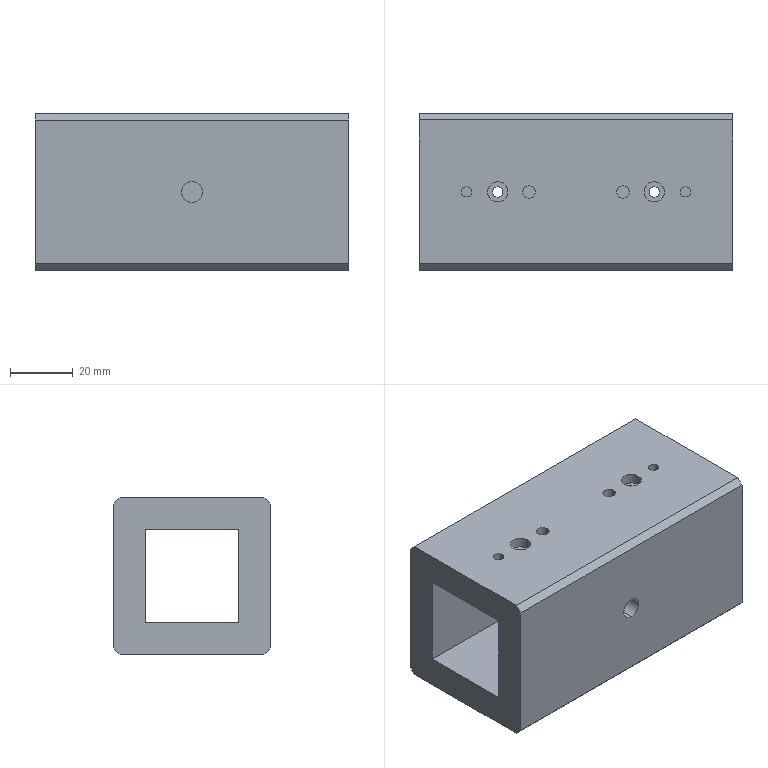Part | SolidWorks | features HoleWzd 7, Chamfer 1, Extrusion 1, ICE 1 | 1 solid | 44 faces | box 100 x 50 x 50 mm | volume 157737 mm3 | cylinder 26 | plane 18 | commonest cylinder face diameters 3.3 x12 6.5 x8 4 x4 6.8 x2
STEP:
#1=CARTESIAN_POINT('',(-26.65,0.,40.));
#2=VERTEX_POINT('',#1);
#3=CARTESIAN_POINT('',(-23.35,0.,40.));
#4=VERTEX_POINT('',#3);
#5=CARTESIAN_POINT('',(-25.,0.,40.));
#6=DIRECTION('',(0.,0.,1.));
#7=DIRECTION('',(0.,-1.,0.));
#8=AXIS2_PLACEMENT_3D('',#5,#6,#7);
#9=CIRCLE('',#8,1.65);
#10=EDGE_CURVE('',#2,#4,#9,.T.);
#11=ORIENTED_EDGE('',*,*,#10,.F.);
#12=CARTESIAN_POINT('',(-26.65,0.,46.6));
#13=VERTEX_POINT('',#12);
#14=CARTESIAN_POINT('',(-26.65,0.,46.6));
#15=DIRECTION('',(0.,0.,1.));
#16=VECTOR('',#15,1000.);
#17=LINE('',#14,#16);
#18=EDGE_CURVE('',#2,#13,#17,.T.);
#19=ORIENTED_EDGE('',*,*,#18,.T.);
#20=CARTESIAN_POINT('',(-23.35,0.,46.6));
#21=VERTEX_POINT('',#20);
#22=CARTESIAN_POINT('',(-25.,0.,46.6));
#23=DIRECTION('',(0.,0.,1.));
#24=DIRECTION('',(1.,0.,0.));
#25=AXIS2_PLACEMENT_3D('',#22,#23,#24);
#26=CIRCLE('',#25,1.65);
#27=EDGE_CURVE('',#13,#21,#26,.T.);
#28=ORIENTED_EDGE('',*,*,#27,.T.);
#29=CARTESIAN_POINT('',(-23.35,0.,46.6));
#30=DIRECTION('',(0.,0.,1.));
#31=VECTOR('',#30,1000.);
#32=LINE('',#29,#31);
#33=EDGE_CURVE('',#4,#21,#32,.T.);
#34=ORIENTED_EDGE('',*,*,#33,.F.);
#35=EDGE_LOOP('',(#11,#19,#28,#34));
#36=FACE_OUTER_BOUND('',#35,.T.);
#37=CARTESIAN_POINT('',(-25.,0.,46.6));
#38=DIRECTION('',(0.,0.,1.));
#39=DIRECTION('',(1.,0.,0.));
#40=AXIS2_PLACEMENT_3D('',#37,#38,#39);
#41=CYLINDRICAL_SURFACE('',#40,1.65);
#42=ADVANCED_FACE('',(#36),#41,.F.);
#43=CARTESIAN_POINT('',(23.35,0.,40.));
#44=VERTEX_POINT('',#43);
#45=CARTESIAN_POINT('',(26.65,0.,40.));
#46=VERTEX_POINT('',#45);
#47=CARTESIAN_POINT('',(25.,0.,40.));
#48=DIRECTION('',(0.,0.,1.));
#49=DIRECTION('',(0.,-1.,0.));
#50=AXIS2_PLACEMENT_3D('',#47,#48,#49);
#51=CIRCLE('',#50,1.65);
#52=EDGE_CURVE('',#44,#46,#51,.T.);
#53=ORIENTED_EDGE('',*,*,#52,.F.);
#54=CARTESIAN_POINT('',(23.35,0.,46.6));
#55=VERTEX_POINT('',#54);
#56=CARTESIAN_POINT('',(23.35,0.,46.6));
#57=DIRECTION('',(0.,0.,1.));
#58=VECTOR('',#57,1000.);
#59=LINE('',#56,#58);
#60=EDGE_CURVE('',#44,#55,#59,.T.);
#61=ORIENTED_EDGE('',*,*,#60,.T.);
#62=CARTESIAN_POINT('',(26.65,0.,46.6));
#63=VERTEX_POINT('',#62);
#64=CARTESIAN_POINT('',(25.,0.,46.6));
#65=DIRECTION('',(0.,0.,1.));
#66=DIRECTION('',(1.,0.,0.));
#67=AXIS2_PLACEMENT_3D('',#64,#65,#66);
#68=CIRCLE('',#67,1.65);
#69=EDGE_CURVE('',#55,#63,#68,.T.);
#70=ORIENTED_EDGE('',*,*,#69,.T.);
#71=CARTESIAN_POINT('',(26.65,0.,46.6));
#72=DIRECTION('',(0.,0.,1.));
#73=VECTOR('',#72,1000.);
#74=LINE('',#71,#73);
#75=EDGE_CURVE('',#46,#63,#74,.T.);
#76=ORIENTED_EDGE('',*,*,#75,.F.);
#77=EDGE_LOOP('',(#53,#61,#70,#76));
#78=FACE_OUTER_BOUND('',#77,.T.);
#79=CARTESIAN_POINT('',(25.,0.,46.6));
#80=DIRECTION('',(0.,0.,1.));
#81=DIRECTION('',(1.,0.,0.));
#82=AXIS2_PLACEMENT_3D('',#79,#80,#81);
#83=CYLINDRICAL_SURFACE('',#82,1.65);
#84=ADVANCED_FACE('',(#78),#83,.F.);
#85=CARTESIAN_POINT('',(26.65,0.,10.));
#86=VERTEX_POINT('',#85);
#87=CARTESIAN_POINT('',(23.35,0.,10.));
#88=VERTEX_POINT('',#87);
#89=CARTESIAN_POINT('',(25.,0.,10.));
#90=DIRECTION('',(0.,0.,-1.));
#91=DIRECTION('',(-1.,0.,0.));
#92=AXIS2_PLACEMENT_3D('',#89,#90,#91);
#93=CIRCLE('',#92,1.65);
#94=EDGE_CURVE('',#86,#88,#93,.T.);
#95=ORIENTED_EDGE('',*,*,#94,.F.);
#96=CARTESIAN_POINT('',(26.65,0.,3.4));
#97=VERTEX_POINT('',#96);
#98=CARTESIAN_POINT('',(26.65,0.,3.4));
#99=DIRECTION('',(0.,0.,-1.));
#100=VECTOR('',#99,1000.);
#101=LINE('',#98,#100);
#102=EDGE_CURVE('',#86,#97,#101,.T.);
#103=ORIENTED_EDGE('',*,*,#102,.T.);
#104=CARTESIAN_POINT('',(23.35,0.,3.4));
#105=VERTEX_POINT('',#104);
#106=CARTESIAN_POINT('',(25.,0.,3.4));
#107=DIRECTION('',(0.,0.,-1.));
#108=DIRECTION('',(-1.,0.,0.));
#109=AXIS2_PLACEMENT_3D('',#106,#107,#108);
#110=CIRCLE('',#109,1.65);
#111=EDGE_CURVE('',#97,#105,#110,.T.);
#112=ORIENTED_EDGE('',*,*,#111,.T.);
#113=CARTESIAN_POINT('',(23.35,0.,3.4));
#114=DIRECTION('',(0.,0.,-1.));
#115=VECTOR('',#114,1000.);
#116=LINE('',#113,#115);
#117=EDGE_CURVE('',#88,#105,#116,.T.);
#118=ORIENTED_EDGE('',*,*,#117,.F.);
#119=EDGE_LOOP('',(#95,#103,#112,#118));
#120=FACE_OUTER_BOUND('',#119,.T.);
#121=CARTESIAN_POINT('',(25.,0.,3.4));
#122=DIRECTION('',(0.,0.,-1.));
#123=DIRECTION('',(-1.,0.,0.));
#124=AXIS2_PLACEMENT_3D('',#121,#122,#123);
#125=CYLINDRICAL_SURFACE('',#124,1.65);
#126=ADVANCED_FACE('',(#120),#125,.F.);
#127=CARTESIAN_POINT('',(-23.35,0.,10.));
#128=VERTEX_POINT('',#127);
#129=CARTESIAN_POINT('',(-26.65,0.,10.));
#130=VERTEX_POINT('',#129);
#131=CARTESIAN_POINT('',(-25.,0.,10.));
#132=DIRECTION('',(0.,0.,-1.));
#133=DIRECTION('',(-1.,0.,0.));
#134=AXIS2_PLACEMENT_3D('',#131,#132,#133);
#135=CIRCLE('',#134,1.65);
#136=EDGE_CURVE('',#128,#130,#135,.T.);
#137=ORIENTED_EDGE('',*,*,#136,.F.);
#138=CARTESIAN_POINT('',(-23.35,0.,3.4));
#139=VERTEX_POINT('',#138);
#140=CARTESIAN_POINT('',(-23.35,0.,3.4));
#141=DIRECTION('',(0.,0.,-1.));
#142=VECTOR('',#141,1000.);
#143=LINE('',#140,#142);
#144=EDGE_CURVE('',#128,#139,#143,.T.);
#145=ORIENTED_EDGE('',*,*,#144,.T.);
#146=CARTESIAN_POINT('',(-26.65,0.,3.4));
#147=VERTEX_POINT('',#146);
#148=CARTESIAN_POINT('',(-25.,0.,3.4));
#149=DIRECTION('',(0.,0.,-1.));
#150=DIRECTION('',(-1.,0.,0.));
#151=AXIS2_PLACEMENT_3D('',#148,#149,#150);
#152=CIRCLE('',#151,1.65);
#153=EDGE_CURVE('',#139,#147,#152,.T.);
#154=ORIENTED_EDGE('',*,*,#153,.T.);
#155=CARTESIAN_POINT('',(-26.65,0.,3.4));
#156=DIRECTION('',(0.,0.,-1.));
#157=VECTOR('',#156,1000.);
#158=LINE('',#155,#157);
#159=EDGE_CURVE('',#130,#147,#158,.T.);
#160=ORIENTED_EDGE('',*,*,#159,.F.);
#161=EDGE_LOOP('',(#137,#145,#154,#160));
#162=FACE_OUTER_BOUND('',#161,.T.);
#163=CARTESIAN_POINT('',(-25.,0.,3.4));
#164=DIRECTION('',(0.,0.,-1.));
#165=DIRECTION('',(-1.,0.,0.));
#166=AXIS2_PLACEMENT_3D('',#163,#164,#165);
#167=CYLINDRICAL_SURFACE('',#166,1.65);
#168=ADVANCED_FACE('',(#162),#167,.F.);
#169=CARTESIAN_POINT('',(0.,-15.,28.4));
#170=VERTEX_POINT('',#169);
#171=CARTESIAN_POINT('',(0.,-15.,21.6));
#172=VERTEX_POINT('',#171);
#173=CARTESIAN_POINT('',(0.,-15.,25.));
#174=DIRECTION('',(0.,-1.,0.));
#175=DIRECTION('',(1.,0.,0.));
#176=AXIS2_PLACEMENT_3D('',#173,#174,#175);
#177=CIRCLE('',#176,3.4);
#178=EDGE_CURVE('',#170,#172,#177,.T.);
#179=ORIENTED_EDGE('',*,*,#178,.F.);
#180=CARTESIAN_POINT('',(0.,-25.,28.4));
#181=VERTEX_POINT('',#180);
#182=CARTESIAN_POINT('',(0.,-25.,28.4));
#183=DIRECTION('',(0.,-1.,0.));
#184=VECTOR('',#183,1000.);
#185=LINE('',#182,#184);
#186=EDGE_CURVE('',#170,#181,#185,.T.);
#187=ORIENTED_EDGE('',*,*,#186,.T.);
#188=CARTESIAN_POINT('',(0.,-25.,21.6));
#189=VERTEX_POINT('',#188);
#190=CARTESIAN_POINT('',(0.,-25.,25.));
#191=DIRECTION('',(0.,-1.,0.));
#192=DIRECTION('',(0.,0.,-1.));
#193=AXIS2_PLACEMENT_3D('',#190,#191,#192);
#194=CIRCLE('',#193,3.4);
#195=EDGE_CURVE('',#181,#189,#194,.T.);
#196=ORIENTED_EDGE('',*,*,#195,.T.);
#197=CARTESIAN_POINT('',(0.,-25.,21.6));
#198=DIRECTION('',(0.,-1.,0.));
#199=VECTOR('',#198,1000.);
#200=LINE('',#197,#199);
#201=EDGE_CURVE('',#172,#189,#200,.T.);
#202=ORIENTED_EDGE('',*,*,#201,.F.);
#203=EDGE_LOOP('',(#179,#187,#196,#202));
#204=FACE_OUTER_BOUND('',#203,.T.);
#205=CARTESIAN_POINT('',(0.,-25.,25.));
#206=DIRECTION('',(0.,-1.,0.));
#207=DIRECTION('',(0.,0.,-1.));
#208=AXIS2_PLACEMENT_3D('',#205,#206,#207);
#209=CYLINDRICAL_SURFACE('',#208,3.4);
#210=ADVANCED_FACE('',(#204),#209,.F.);
#211=CARTESIAN_POINT('',(13.,0.,40.));
#212=VERTEX_POINT('',#211);
#213=CARTESIAN_POINT('',(17.,0.,40.));
#214=VERTEX_POINT('',#213);
#215=CARTESIAN_POINT('',(15.,0.,40.));
#216=DIRECTION('',(0.,0.,1.));
#217=DIRECTION('',(0.,-1.,0.));
#218=AXIS2_PLACEMENT_3D('',#215,#216,#217);
#219=CIRCLE('',#218,2.);
#220=EDGE_CURVE('',#212,#214,#219,.T.);
#221=ORIENTED_EDGE('',*,*,#220,.F.);
#222=CARTESIAN_POINT('',(13.,0.,50.));
#223=VERTEX_POINT('',#222);
#224=CARTESIAN_POINT('',(13.,0.,50.));
#225=DIRECTION('',(0.,0.,1.));
#226=VECTOR('',#225,1000.);
#227=LINE('',#224,#226);
#228=EDGE_CURVE('',#212,#223,#227,.T.);
#229=ORIENTED_EDGE('',*,*,#228,.T.);
#230=CARTESIAN_POINT('',(17.,0.,50.));
#231=VERTEX_POINT('',#230);
#232=CARTESIAN_POINT('',(15.,0.,50.));
#233=DIRECTION('',(0.,0.,1.));
#234=DIRECTION('',(1.,0.,0.));
#235=AXIS2_PLACEMENT_3D('',#232,#233,#234);
#236=CIRCLE('',#235,2.);
#237=EDGE_CURVE('',#223,#231,#236,.T.);
#238=ORIENTED_EDGE('',*,*,#237,.T.);
#239=CARTESIAN_POINT('',(17.,0.,50.));
#240=DIRECTION('',(0.,0.,1.));
#241=VECTOR('',#240,1000.);
#242=LINE('',#239,#241);
#243=EDGE_CURVE('',#214,#231,#242,.T.);
#244=ORIENTED_EDGE('',*,*,#243,.F.);
#245=EDGE_LOOP('',(#221,#229,#238,#244));
#246=FACE_OUTER_BOUND('',#245,.T.);
#247=CARTESIAN_POINT('',(15.,0.,50.));
#248=DIRECTION('',(0.,0.,1.));
#249=DIRECTION('',(1.,0.,0.));
#250=AXIS2_PLACEMENT_3D('',#247,#248,#249);
#251=CYLINDRICAL_SURFACE('',#250,2.);
#252=ADVANCED_FACE('',(#246),#251,.F.);
#253=CARTESIAN_POINT('',(-17.,0.,40.));
#254=VERTEX_POINT('',#253);
#255=CARTESIAN_POINT('',(-13.,0.,40.));
#256=VERTEX_POINT('',#255);
#257=CARTESIAN_POINT('',(-15.,0.,40.));
#258=DIRECTION('',(0.,0.,1.));
#259=DIRECTION('',(0.,-1.,0.));
#260=AXIS2_PLACEMENT_3D('',#257,#258,#259);
#261=CIRCLE('',#260,2.);
#262=EDGE_CURVE('',#254,#256,#261,.T.);
#263=ORIENTED_EDGE('',*,*,#262,.F.);
#264=CARTESIAN_POINT('',(-17.,0.,50.));
#265=VERTEX_POINT('',#264);
#266=CARTESIAN_POINT('',(-17.,0.,50.));
#267=DIRECTION('',(0.,0.,1.));
#268=VECTOR('',#267,1000.);
#269=LINE('',#266,#268);
#270=EDGE_CURVE('',#254,#265,#269,.T.);
#271=ORIENTED_EDGE('',*,*,#270,.T.);
#272=CARTESIAN_POINT('',(-13.,0.,50.));
#273=VERTEX_POINT('',#272);
#274=CARTESIAN_POINT('',(-15.,0.,50.));
#275=DIRECTION('',(0.,0.,1.));
#276=DIRECTION('',(1.,0.,0.));
#277=AXIS2_PLACEMENT_3D('',#274,#275,#276);
#278=CIRCLE('',#277,2.);
#279=EDGE_CURVE('',#265,#273,#278,.T.);
#280=ORIENTED_EDGE('',*,*,#279,.T.);
#281=CARTESIAN_POINT('',(-13.,0.,50.));
#282=DIRECTION('',(0.,0.,1.));
#283=VECTOR('',#282,1000.);
#284=LINE('',#281,#283);
#285=EDGE_CURVE('',#256,#273,#284,.T.);
#286=ORIENTED_EDGE('',*,*,#285,.F.);
#287=EDGE_LOOP('',(#263,#271,#280,#286));
#288=FACE_OUTER_BOUND('',#287,.T.);
#289=CARTESIAN_POINT('',(-15.,0.,50.));
#290=DIRECTION('',(0.,0.,1.));
#291=DIRECTION('',(1.,0.,0.));
#292=AXIS2_PLACEMENT_3D('',#289,#290,#291);
#293=CYLINDRICAL_SURFACE('',#292,2.);
#294=ADVANCED_FACE('',(#288),#293,.F.);
#295=CARTESIAN_POINT('',(-36.65,0.,40.));
#296=VERTEX_POINT('',#295);
#297=CARTESIAN_POINT('',(-33.35,0.,40.));
#298=VERTEX_POINT('',#297);
#299=CARTESIAN_POINT('',(-35.,0.,40.));
#300=DIRECTION('',(0.,0.,1.));
#301=DIRECTION('',(0.,-1.,0.));
#302=AXIS2_PLACEMENT_3D('',#299,#300,#301);
#303=CIRCLE('',#302,1.65);
#304=EDGE_CURVE('',#296,#298,#303,.T.);
#305=ORIENTED_EDGE('',*,*,#304,.F.);
#306=CARTESIAN_POINT('',(-36.65,0.,50.));
#307=VERTEX_POINT('',#306);
#308=CARTESIAN_POINT('',(-36.65,0.,50.));
#309=DIRECTION('',(0.,0.,1.));
#310=VECTOR('',#309,1000.);
#311=LINE('',#308,#310);
#312=EDGE_CURVE('',#296,#307,#311,.T.);
#313=ORIENTED_EDGE('',*,*,#312,.T.);
#314=CARTESIAN_POINT('',(-33.35,0.,50.));
#315=VERTEX_POINT('',#314);
#316=CARTESIAN_POINT('',(-35.,0.,50.));
#317=DIRECTION('',(0.,0.,1.));
#318=DIRECTION('',(1.,0.,0.));
#319=AXIS2_PLACEMENT_3D('',#316,#317,#318);
#320=CIRCLE('',#319,1.65);
#321=EDGE_CURVE('',#307,#315,#320,.T.);
#322=ORIENTED_EDGE('',*,*,#321,.T.);
#323=CARTESIAN_POINT('',(-33.35,0.,50.));
#324=DIRECTION('',(0.,0.,1.));
#325=VECTOR('',#324,1000.);
#326=LINE('',#323,#325);
#327=EDGE_CURVE('',#298,#315,#326,.T.);
#328=ORIENTED_EDGE('',*,*,#327,.F.);
#329=EDGE_LOOP('',(#305,#313,#322,#328));
#330=FACE_OUTER_BOUND('',#329,.T.);
#331=CARTESIAN_POINT('',(-35.,0.,50.));
#332=DIRECTION('',(0.,0.,1.));
#333=DIRECTION('',(1.,0.,0.));
#334=AXIS2_PLACEMENT_3D('',#331,#332,#333);
#335=CYLINDRICAL_SURFACE('',#334,1.65);
#336=ADVANCED_FACE('',(#330),#335,.F.);
#337=CARTESIAN_POINT('',(33.35,0.,40.));
#338=VERTEX_POINT('',#337);
#339=CARTESIAN_POINT('',(36.65,0.,40.));
#340=VERTEX_POINT('',#339);
#341=CARTESIAN_POINT('',(35.,0.,40.));
#342=DIRECTION('',(0.,0.,1.));
#343=DIRECTION('',(0.,-1.,0.));
#344=AXIS2_PLACEMENT_3D('',#341,#342,#343);
#345=CIRCLE('',#344,1.65);
#346=EDGE_CURVE('',#338,#340,#345,.T.);
#347=ORIENTED_EDGE('',*,*,#346,.F.);
#348=CARTESIAN_POINT('',(33.35,0.,50.));
#349=VERTEX_POINT('',#348);
#350=CARTESIAN_POINT('',(33.35,0.,50.));
#351=DIRECTION('',(0.,0.,1.));
#352=VECTOR('',#351,1000.);
#353=LINE('',#350,#352);
#354=EDGE_CURVE('',#338,#349,#353,.T.);
#355=ORIENTED_EDGE('',*,*,#354,.T.);
#356=CARTESIAN_POINT('',(36.65,0.,50.));
#357=VERTEX_POINT('',#356);
#358=CARTESIAN_POINT('',(35.,0.,50.));
#359=DIRECTION('',(0.,0.,1.));
#360=DIRECTION('',(1.,0.,0.));
#361=AXIS2_PLACEMENT_3D('',#358,#359,#360);
#362=CIRCLE('',#361,1.65);
#363=EDGE_CURVE('',#349,#357,#362,.T.);
#364=ORIENTED_EDGE('',*,*,#363,.T.);
#365=CARTESIAN_POINT('',(36.65,0.,50.));
#366=DIRECTION('',(0.,0.,1.));
#367=VECTOR('',#366,1000.);
#368=LINE('',#365,#367);
#369=EDGE_CURVE('',#340,#357,#368,.T.);
#370=ORIENTED_EDGE('',*,*,#369,.F.);
#371=EDGE_LOOP('',(#347,#355,#364,#370));
#372=FACE_OUTER_BOUND('',#371,.T.);
#373=CARTESIAN_POINT('',(35.,0.,50.));
#374=DIRECTION('',(0.,0.,1.));
#375=DIRECTION('',(1.,0.,0.));
#376=AXIS2_PLACEMENT_3D('',#373,#374,#375);
#377=CYLINDRICAL_SURFACE('',#376,1.65);
#378=ADVANCED_FACE('',(#372),#377,.F.);
#379=CARTESIAN_POINT('',(-28.25,0.,46.6));
#380=VERTEX_POINT('',#379);
#381=CARTESIAN_POINT('',(-21.75,0.,46.6));
#382=VERTEX_POINT('',#381);
#383=CARTESIAN_POINT('',(-25.,0.,46.6));
#384=DIRECTION('',(0.,0.,1.));
#385=DIRECTION('',(1.,0.,0.));
#386=AXIS2_PLACEMENT_3D('',#383,#384,#385);
#387=CIRCLE('',#386,3.25);
#388=EDGE_CURVE('',#380,#382,#387,.T.);
#389=ORIENTED_EDGE('',*,*,#388,.F.);
#390=CARTESIAN_POINT('',(-28.25,0.,50.));
#391=VERTEX_POINT('',#390);
#392=CARTESIAN_POINT('',(-28.25,0.,50.));
#393=DIRECTION('',(0.,0.,1.));
#394=VECTOR('',#393,1000.);
#395=LINE('',#392,#394);
#396=EDGE_CURVE('',#380,#391,#395,.T.);
#397=ORIENTED_EDGE('',*,*,#396,.T.);
#398=CARTESIAN_POINT('',(-21.75,0.,50.));
#399=VERTEX_POINT('',#398);
#400=CARTESIAN_POINT('',(-25.,0.,50.));
#401=DIRECTION('',(0.,0.,1.));
#402=DIRECTION('',(1.,0.,0.));
#403=AXIS2_PLACEMENT_3D('',#400,#401,#402);
#404=CIRCLE('',#403,3.25);
#405=EDGE_CURVE('',#391,#399,#404,.T.);
#406=ORIENTED_EDGE('',*,*,#405,.T.);
#407=CARTESIAN_POINT('',(-21.75,0.,50.));
#408=DIRECTION('',(0.,0.,1.));
#409=VECTOR('',#408,1000.);
#410=LINE('',#407,#409);
#411=EDGE_CURVE('',#382,#399,#410,.T.);
#412=ORIENTED_EDGE('',*,*,#411,.F.);
#413=EDGE_LOOP('',(#389,#397,#406,#412));
#414=FACE_OUTER_BOUND('',#413,.T.);
#415=CARTESIAN_POINT('',(-25.,0.,50.));
#416=DIRECTION('',(0.,0.,1.));
#417=DIRECTION('',(1.,0.,0.));
#418=AXIS2_PLACEMENT_3D('',#415,#416,#417);
#419=CYLINDRICAL_SURFACE('',#418,3.25);
#420=ADVANCED_FACE('',(#414),#419,.F.);
#421=CARTESIAN_POINT('',(21.75,0.,46.6));
#422=VERTEX_POINT('',#421);
#423=CARTESIAN_POINT('',(28.25,0.,46.6));
#424=VERTEX_POINT('',#423);
#425=CARTESIAN_POINT('',(25.,0.,46.6));
#426=DIRECTION('',(0.,0.,1.));
#427=DIRECTION('',(1.,0.,0.));
#428=AXIS2_PLACEMENT_3D('',#425,#426,#427);
#429=CIRCLE('',#428,3.25);
#430=EDGE_CURVE('',#422,#424,#429,.T.);
#431=ORIENTED_EDGE('',*,*,#430,.F.);
#432=CARTESIAN_POINT('',(21.75,0.,50.));
#433=VERTEX_POINT('',#432);
#434=CARTESIAN_POINT('',(21.75,0.,50.));
#435=DIRECTION('',(0.,0.,1.));
#436=VECTOR('',#435,1000.);
#437=LINE('',#434,#436);
#438=EDGE_CURVE('',#422,#433,#437,.T.);
#439=ORIENTED_EDGE('',*,*,#438,.T.);
#440=CARTESIAN_POINT('',(28.25,0.,50.));
#441=VERTEX_POINT('',#440);
#442=CARTESIAN_POINT('',(25.,0.,50.));
#443=DIRECTION('',(0.,0.,1.));
#444=DIRECTION('',(1.,0.,0.));
#445=AXIS2_PLACEMENT_3D('',#442,#443,#444);
#446=CIRCLE('',#445,3.25);
#447=EDGE_CURVE('',#433,#441,#446,.T.);
#448=ORIENTED_EDGE('',*,*,#447,.T.);
#449=CARTESIAN_POINT('',(28.25,0.,50.));
#450=DIRECTION('',(0.,0.,1.));
#451=VECTOR('',#450,1000.);
#452=LINE('',#449,#451);
#453=EDGE_CURVE('',#424,#441,#452,.T.);
#454=ORIENTED_EDGE('',*,*,#453,.F.);
#455=EDGE_LOOP('',(#431,#439,#448,#454));
#456=FACE_OUTER_BOUND('',#455,.T.);
#457=CARTESIAN_POINT('',(25.,0.,50.));
#458=DIRECTION('',(0.,0.,1.));
#459=DIRECTION('',(1.,0.,0.));
#460=AXIS2_PLACEMENT_3D('',#457,#458,#459);
#461=CYLINDRICAL_SURFACE('',#460,3.25);
#462=ADVANCED_FACE('',(#456),#461,.F.);
#463=CARTESIAN_POINT('',(28.25,0.,3.4));
#464=VERTEX_POINT('',#463);
#465=CARTESIAN_POINT('',(21.75,0.,3.4));
#466=VERTEX_POINT('',#465);
#467=CARTESIAN_POINT('',(25.,0.,3.4));
#468=DIRECTION('',(0.,0.,-1.));
#469=DIRECTION('',(-1.,0.,0.));
#470=AXIS2_PLACEMENT_3D('',#467,#468,#469);
#471=CIRCLE('',#470,3.25);
#472=EDGE_CURVE('',#464,#466,#471,.T.);
#473=ORIENTED_EDGE('',*,*,#472,.F.);
#474=CARTESIAN_POINT('',(28.25,0.,0.));
#475=VERTEX_POINT('',#474);
#476=CARTESIAN_POINT('',(28.25,0.,0.));
#477=DIRECTION('',(0.,0.,-1.));
#478=VECTOR('',#477,1000.);
#479=LINE('',#476,#478);
#480=EDGE_CURVE('',#464,#475,#479,.T.);
#481=ORIENTED_EDGE('',*,*,#480,.T.);
#482=CARTESIAN_POINT('',(21.75,0.,0.));
#483=VERTEX_POINT('',#482);
#484=CARTESIAN_POINT('',(25.,0.,0.));
#485=DIRECTION('',(0.,0.,-1.));
#486=DIRECTION('',(-1.,0.,0.));
#487=AXIS2_PLACEMENT_3D('',#484,#485,#486);
#488=CIRCLE('',#487,3.25);
#489=EDGE_CURVE('',#475,#483,#488,.T.);
#490=ORIENTED_EDGE('',*,*,#489,.T.);
#491=CARTESIAN_POINT('',(21.75,0.,0.));
#492=DIRECTION('',(0.,0.,-1.));
#493=VECTOR('',#492,1000.);
#494=LINE('',#491,#493);
#495=EDGE_CURVE('',#466,#483,#494,.T.);
#496=ORIENTED_EDGE('',*,*,#495,.F.);
#497=EDGE_LOOP('',(#473,#481,#490,#496));
#498=FACE_OUTER_BOUND('',#497,.T.);
#499=CARTESIAN_POINT('',(25.,0.,0.));
#500=DIRECTION('',(0.,0.,-1.));
#501=DIRECTION('',(-1.,0.,0.));
#502=AXIS2_PLACEMENT_3D('',#499,#500,#501);
#503=CYLINDRICAL_SURFACE('',#502,3.25);
#504=ADVANCED_FACE('',(#498),#503,.F.);
#505=CARTESIAN_POINT('',(-21.75,0.,3.4));
#506=VERTEX_POINT('',#505);
#507=CARTESIAN_POINT('',(-28.25,0.,3.4));
#508=VERTEX_POINT('',#507);
#509=CARTESIAN_POINT('',(-25.,0.,3.4));
#510=DIRECTION('',(0.,0.,-1.));
#511=DIRECTION('',(-1.,0.,0.));
#512=AXIS2_PLACEMENT_3D('',#509,#510,#511);
#513=CIRCLE('',#512,3.25);
#514=EDGE_CURVE('',#506,#508,#513,.T.);
#515=ORIENTED_EDGE('',*,*,#514,.F.);
#516=CARTESIAN_POINT('',(-21.75,0.,0.));
#517=VERTEX_POINT('',#516);
#518=CARTESIAN_POINT('',(-21.75,0.,0.));
#519=DIRECTION('',(0.,0.,-1.));
#520=VECTOR('',#519,1000.);
#521=LINE('',#518,#520);
#522=EDGE_CURVE('',#506,#517,#521,.T.);
#523=ORIENTED_EDGE('',*,*,#522,.T.);
#524=CARTESIAN_POINT('',(-28.25,0.,0.));
#525=VERTEX_POINT('',#524);
#526=CARTESIAN_POINT('',(-25.,0.,0.));
#527=DIRECTION('',(0.,0.,-1.));
#528=DIRECTION('',(-1.,0.,0.));
#529=AXIS2_PLACEMENT_3D('',#526,#527,#528);
#530=CIRCLE('',#529,3.25);
#531=EDGE_CURVE('',#517,#525,#530,.T.);
#532=ORIENTED_EDGE('',*,*,#531,.T.);
#533=CARTESIAN_POINT('',(-28.25,0.,0.));
#534=DIRECTION('',(0.,0.,-1.));
#535=VECTOR('',#534,1000.);
#536=LINE('',#533,#535);
#537=EDGE_CURVE('',#508,#525,#536,.T.);
#538=ORIENTED_EDGE('',*,*,#537,.F.);
#539=EDGE_LOOP('',(#515,#523,#532,#538));
#540=FACE_OUTER_BOUND('',#539,.T.);
#541=CARTESIAN_POINT('',(-25.,0.,0.));
#542=DIRECTION('',(0.,0.,-1.));
#543=DIRECTION('',(-1.,0.,0.));
#544=AXIS2_PLACEMENT_3D('',#541,#542,#543);
#545=CYLINDRICAL_SURFACE('',#544,3.25);
#546=ADVANCED_FACE('',(#540),#545,.F.);
#547=CARTESIAN_POINT('',(50.,-15.,40.));
#548=VERTEX_POINT('',#547);
#549=CARTESIAN_POINT('',(50.,-15.,10.));
#550=VERTEX_POINT('',#549);
#551=CARTESIAN_POINT('',(50.,-15.,40.));
#552=DIRECTION('',(0.,0.,-1.));
#553=VECTOR('',#552,1000.);
#554=LINE('',#551,#553);
#555=EDGE_CURVE('',#548,#550,#554,.T.);
#556=ORIENTED_EDGE('',*,*,#555,.F.);
#557=CARTESIAN_POINT('',(50.,15.,40.));
#558=VERTEX_POINT('',#557);
#559=CARTESIAN_POINT('',(50.,15.,40.));
#560=DIRECTION('',(0.,-1.,0.));
#561=VECTOR('',#560,1000.);
#562=LINE('',#559,#561);
#563=EDGE_CURVE('',#558,#548,#562,.T.);
#564=ORIENTED_EDGE('',*,*,#563,.F.);
#565=CARTESIAN_POINT('',(50.,15.,10.));
#566=VERTEX_POINT('',#565);
#567=CARTESIAN_POINT('',(50.,15.,40.));
#568=DIRECTION('',(0.,0.,1.));
#569=VECTOR('',#568,1000.);
#570=LINE('',#567,#569);
#571=EDGE_CURVE('',#566,#558,#570,.T.);
#572=ORIENTED_EDGE('',*,*,#571,.F.);
#573=CARTESIAN_POINT('',(50.,15.,10.));
#574=DIRECTION('',(0.,1.,0.));
#575=VECTOR('',#574,1000.);
#576=LINE('',#573,#575);
#577=EDGE_CURVE('',#550,#566,#576,.T.);
#578=ORIENTED_EDGE('',*,*,#577,.F.);
#579=EDGE_LOOP('',(#556,#564,#572,#578));
#580=FACE_BOUND('',#579,.T.);
#581=CARTESIAN_POINT('',(50.,-23.,50.));
#582=VERTEX_POINT('',#581);
#583=CARTESIAN_POINT('',(50.,23.,50.));
#584=VERTEX_POINT('',#583);
#585=CARTESIAN_POINT('',(50.,25.,50.));
#586=DIRECTION('',(0.,1.,0.));
#587=VECTOR('',#586,1000.);
#588=LINE('',#585,#587);
#589=EDGE_CURVE('',#582,#584,#588,.T.);
#590=ORIENTED_EDGE('',*,*,#589,.F.);
#591=CARTESIAN_POINT('',(50.,-25.,48.));
#592=VERTEX_POINT('',#591);
#593=CARTESIAN_POINT('',(50.,-23.,50.));
#594=DIRECTION('',(0.,-0.7071,-0.7071));
#595=VECTOR('',#594,1000.);
#596=LINE('',#593,#595);
#597=EDGE_CURVE('',#582,#592,#596,.T.);
#598=ORIENTED_EDGE('',*,*,#597,.T.);
#599=CARTESIAN_POINT('',(50.,-25.,2.));
#600=VERTEX_POINT('',#599);
#601=CARTESIAN_POINT('',(50.,-25.,50.));
#602=DIRECTION('',(0.,0.,-1.));
#603=VECTOR('',#602,1000.);
#604=LINE('',#601,#603);
#605=EDGE_CURVE('',#592,#600,#604,.T.);
#606=ORIENTED_EDGE('',*,*,#605,.T.);
#607=CARTESIAN_POINT('',(50.,-23.,0.));
#608=VERTEX_POINT('',#607);
#609=CARTESIAN_POINT('',(50.,-25.,2.));
#610=DIRECTION('',(0.,0.7071,-0.7071));
#611=VECTOR('',#610,1000.);
#612=LINE('',#609,#611);
#613=EDGE_CURVE('',#600,#608,#612,.T.);
#614=ORIENTED_EDGE('',*,*,#613,.T.);
#615=CARTESIAN_POINT('',(50.,23.,0.));
#616=VERTEX_POINT('',#615);
#617=CARTESIAN_POINT('',(50.,25.,0.));
#618=DIRECTION('',(0.,1.,0.));
#619=VECTOR('',#618,1000.);
#620=LINE('',#617,#619);
#621=EDGE_CURVE('',#608,#616,#620,.T.);
#622=ORIENTED_EDGE('',*,*,#621,.T.);
#623=CARTESIAN_POINT('',(50.,25.,2.));
#624=VERTEX_POINT('',#623);
#625=CARTESIAN_POINT('',(50.,25.,2.));
#626=DIRECTION('',(0.,0.7071,0.7071));
#627=VECTOR('',#626,1000.);
#628=LINE('',#625,#627);
#629=EDGE_CURVE('',#616,#624,#628,.T.);
#630=ORIENTED_EDGE('',*,*,#629,.T.);
#631=CARTESIAN_POINT('',(50.,25.,48.));
#632=VERTEX_POINT('',#631);
#633=CARTESIAN_POINT('',(50.,25.,50.));
#634=DIRECTION('',(0.,0.,-1.));
#635=VECTOR('',#634,1000.);
#636=LINE('',#633,#635);
#637=EDGE_CURVE('',#632,#624,#636,.T.);
#638=ORIENTED_EDGE('',*,*,#637,.F.);
#639=CARTESIAN_POINT('',(50.,23.,50.));
#640=DIRECTION('',(0.,-0.7071,0.7071));
#641=VECTOR('',#640,1000.);
#642=LINE('',#639,#641);
#643=EDGE_CURVE('',#632,#584,#642,.T.);
#644=ORIENTED_EDGE('',*,*,#643,.T.);
#645=EDGE_LOOP('',(#590,#598,#606,#614,#622,#630,#638,#644));
#646=FACE_OUTER_BOUND('',#645,.T.);
#647=CARTESIAN_POINT('',(50.,25.,50.));
#648=DIRECTION('',(-1.,0.,0.));
#649=DIRECTION('',(0.,0.,1.));
#650=AXIS2_PLACEMENT_3D('',#647,#648,#649);
#651=PLANE('',#650);
#652=ADVANCED_FACE('',(#580,#646),#651,.F.);
#653=CARTESIAN_POINT('',(-50.,25.,48.));
#654=VERTEX_POINT('',#653);
#655=CARTESIAN_POINT('',(-50.,25.,2.));
#656=VERTEX_POINT('',#655);
#657=CARTESIAN_POINT('',(-50.,25.,50.));
#658=DIRECTION('',(0.,0.,-1.));
#659=VECTOR('',#658,1000.);
#660=LINE('',#657,#659);
#661=EDGE_CURVE('',#654,#656,#660,.T.);
#662=ORIENTED_EDGE('',*,*,#661,.F.);
#663=CARTESIAN_POINT('',(50.,25.,48.));
#664=DIRECTION('',(1.,0.,0.));
#665=VECTOR('',#664,1000.);
#666=LINE('',#663,#665);
#667=EDGE_CURVE('',#654,#632,#666,.T.);
#668=ORIENTED_EDGE('',*,*,#667,.T.);
#669=ORIENTED_EDGE('',*,*,#637,.T.);
#670=CARTESIAN_POINT('',(-50.,25.,2.));
#671=DIRECTION('',(-1.,0.,0.));
#672=VECTOR('',#671,1000.);
#673=LINE('',#670,#672);
#674=EDGE_CURVE('',#624,#656,#673,.T.);
#675=ORIENTED_EDGE('',*,*,#674,.T.);
#676=EDGE_LOOP('',(#662,#668,#669,#675));
#677=FACE_OUTER_BOUND('',#676,.T.);
#678=CARTESIAN_POINT('',(-50.,25.,50.));
#679=DIRECTION('',(0.,-1.,0.));
#680=DIRECTION('',(0.,0.,-1.));
#681=AXIS2_PLACEMENT_3D('',#678,#679,#680);
#682=PLANE('',#681);
#683=ADVANCED_FACE('',(#677),#682,.F.);
#684=CARTESIAN_POINT('',(-50.,15.,10.));
#685=VERTEX_POINT('',#684);
#686=CARTESIAN_POINT('',(-50.,15.,40.));
#687=VERTEX_POINT('',#686);
#688=CARTESIAN_POINT('',(-50.,15.,40.));
#689=DIRECTION('',(0.,0.,1.));
#690=VECTOR('',#689,1000.);
#691=LINE('',#688,#690);
#692=EDGE_CURVE('',#685,#687,#691,.T.);
#693=ORIENTED_EDGE('',*,*,#692,.T.);
#694=CARTESIAN_POINT('',(-50.,-15.,40.));
#695=VERTEX_POINT('',#694);
#696=CARTESIAN_POINT('',(-50.,15.,40.));
#697=DIRECTION('',(0.,-1.,0.));
#698=VECTOR('',#697,1000.);
#699=LINE('',#696,#698);
#700=EDGE_CURVE('',#687,#695,#699,.T.);
#701=ORIENTED_EDGE('',*,*,#700,.T.);
#702=CARTESIAN_POINT('',(-50.,-15.,10.));
#703=VERTEX_POINT('',#702);
#704=CARTESIAN_POINT('',(-50.,-15.,40.));
#705=DIRECTION('',(0.,0.,-1.));
#706=VECTOR('',#705,1000.);
#707=LINE('',#704,#706);
#708=EDGE_CURVE('',#695,#703,#707,.T.);
#709=ORIENTED_EDGE('',*,*,#708,.T.);
#710=CARTESIAN_POINT('',(-50.,15.,10.));
#711=DIRECTION('',(0.,1.,0.));
#712=VECTOR('',#711,1000.);
#713=LINE('',#710,#712);
#714=EDGE_CURVE('',#703,#685,#713,.T.);
#715=ORIENTED_EDGE('',*,*,#714,.T.);
#716=EDGE_LOOP('',(#693,#701,#709,#715));
#717=FACE_BOUND('',#716,.T.);
#718=CARTESIAN_POINT('',(-50.,-25.,48.));
#719=VERTEX_POINT('',#718);
#720=CARTESIAN_POINT('',(-50.,-25.,2.));
#721=VERTEX_POINT('',#720);
#722=CARTESIAN_POINT('',(-50.,-25.,50.));
#723=DIRECTION('',(0.,0.,-1.));
#724=VECTOR('',#723,1000.);
#725=LINE('',#722,#724);
#726=EDGE_CURVE('',#719,#721,#725,.T.);
#727=ORIENTED_EDGE('',*,*,#726,.F.);
#728=CARTESIAN_POINT('',(-50.,-23.,50.));
#729=VERTEX_POINT('',#728);
#730=CARTESIAN_POINT('',(-50.,-23.,50.));
#731=DIRECTION('',(0.,0.7071,0.7071));
#732=VECTOR('',#731,1000.);
#733=LINE('',#730,#732);
#734=EDGE_CURVE('',#719,#729,#733,.T.);
#735=ORIENTED_EDGE('',*,*,#734,.T.);
#736=CARTESIAN_POINT('',(-50.,23.,50.));
#737=VERTEX_POINT('',#736);
#738=CARTESIAN_POINT('',(-50.,25.,50.));
#739=DIRECTION('',(0.,-1.,0.));
#740=VECTOR('',#739,1000.);
#741=LINE('',#738,#740);
#742=EDGE_CURVE('',#737,#729,#741,.T.);
#743=ORIENTED_EDGE('',*,*,#742,.F.);
#744=CARTESIAN_POINT('',(-50.,23.,50.));
#745=DIRECTION('',(0.,0.7071,-0.7071));
#746=VECTOR('',#745,1000.);
#747=LINE('',#744,#746);
#748=EDGE_CURVE('',#737,#654,#747,.T.);
#749=ORIENTED_EDGE('',*,*,#748,.T.);
#750=ORIENTED_EDGE('',*,*,#661,.T.);
#751=CARTESIAN_POINT('',(-50.,23.,0.));
#752=VERTEX_POINT('',#751);
#753=CARTESIAN_POINT('',(-50.,25.,2.));
#754=DIRECTION('',(0.,-0.7071,-0.7071));
#755=VECTOR('',#754,1000.);
#756=LINE('',#753,#755);
#757=EDGE_CURVE('',#656,#752,#756,.T.);
#758=ORIENTED_EDGE('',*,*,#757,.T.);
#759=CARTESIAN_POINT('',(-50.,-23.,0.));
#760=VERTEX_POINT('',#759);
#761=CARTESIAN_POINT('',(-50.,25.,0.));
#762=DIRECTION('',(0.,-1.,0.));
#763=VECTOR('',#762,1000.);
#764=LINE('',#761,#763);
#765=EDGE_CURVE('',#752,#760,#764,.T.);
#766=ORIENTED_EDGE('',*,*,#765,.T.);
#767=CARTESIAN_POINT('',(-50.,-25.,2.));
#768=DIRECTION('',(0.,-0.7071,0.7071));
#769=VECTOR('',#768,1000.);
#770=LINE('',#767,#769);
#771=EDGE_CURVE('',#760,#721,#770,.T.);
#772=ORIENTED_EDGE('',*,*,#771,.T.);
#773=EDGE_LOOP('',(#727,#735,#743,#749,#750,#758,#766,#772));
#774=FACE_OUTER_BOUND('',#773,.T.);
#775=CARTESIAN_POINT('',(-50.,25.,50.));
#776=DIRECTION('',(1.,0.,0.));
#777=DIRECTION('',(0.,1.,0.));
#778=AXIS2_PLACEMENT_3D('',#775,#776,#777);
#779=PLANE('',#778);
#780=ADVANCED_FACE('',(#717,#774),#779,.F.);
#781=CARTESIAN_POINT('',(0.,-25.,25.));
#782=DIRECTION('',(0.,-1.,0.));
#783=DIRECTION('',(0.,0.,-1.));
#784=AXIS2_PLACEMENT_3D('',#781,#782,#783);
#785=CIRCLE('',#784,3.4);
#786=EDGE_CURVE('',#189,#181,#785,.T.);
#787=ORIENTED_EDGE('',*,*,#786,.F.);
#788=ORIENTED_EDGE('',*,*,#195,.F.);
#789=EDGE_LOOP('',(#787,#788));
#790=FACE_BOUND('',#789,.T.);
#791=ORIENTED_EDGE('',*,*,#605,.F.);
#792=CARTESIAN_POINT('',(-50.,-25.,48.));
#793=DIRECTION('',(-1.,0.,0.));
#794=VECTOR('',#793,1000.);
#795=LINE('',#792,#794);
#796=EDGE_CURVE('',#592,#719,#795,.T.);
#797=ORIENTED_EDGE('',*,*,#796,.T.);
#798=ORIENTED_EDGE('',*,*,#726,.T.);
#799=CARTESIAN_POINT('',(-50.,-25.,2.));
#800=DIRECTION('',(1.,0.,0.));
#801=VECTOR('',#800,1000.);
#802=LINE('',#799,#801);
#803=EDGE_CURVE('',#721,#600,#802,.T.);
#804=ORIENTED_EDGE('',*,*,#803,.T.);
#805=EDGE_LOOP('',(#791,#797,#798,#804));
#806=FACE_OUTER_BOUND('',#805,.T.);
#807=CARTESIAN_POINT('',(-50.,-25.,50.));
#808=DIRECTION('',(0.,1.,0.));
#809=DIRECTION('',(0.,0.,1.));
#810=AXIS2_PLACEMENT_3D('',#807,#808,#809);
#811=PLANE('',#810);
#812=ADVANCED_FACE('',(#790,#806),#811,.F.);
#813=CARTESIAN_POINT('',(15.,0.,50.));
#814=DIRECTION('',(0.,0.,1.));
#815=DIRECTION('',(1.,0.,0.));
#816=AXIS2_PLACEMENT_3D('',#813,#814,#815);
#817=CIRCLE('',#816,2.);
#818=EDGE_CURVE('',#231,#223,#817,.T.);
#819=ORIENTED_EDGE('',*,*,#818,.F.);
#820=ORIENTED_EDGE('',*,*,#237,.F.);
#821=EDGE_LOOP('',(#819,#820));
#822=FACE_BOUND('',#821,.T.);
#823=CARTESIAN_POINT('',(-15.,0.,50.));
#824=DIRECTION('',(0.,0.,1.));
#825=DIRECTION('',(1.,0.,0.));
#826=AXIS2_PLACEMENT_3D('',#823,#824,#825);
#827=CIRCLE('',#826,2.);
#828=EDGE_CURVE('',#273,#265,#827,.T.);
#829=ORIENTED_EDGE('',*,*,#828,.F.);
#830=ORIENTED_EDGE('',*,*,#279,.F.);
#831=EDGE_LOOP('',(#829,#830));
#832=FACE_BOUND('',#831,.T.);
#833=CARTESIAN_POINT('',(-35.,0.,50.));
#834=DIRECTION('',(0.,0.,1.));
#835=DIRECTION('',(1.,0.,0.));
#836=AXIS2_PLACEMENT_3D('',#833,#834,#835);
#837=CIRCLE('',#836,1.65);
#838=EDGE_CURVE('',#315,#307,#837,.T.);
#839=ORIENTED_EDGE('',*,*,#838,.F.);
#840=ORIENTED_EDGE('',*,*,#321,.F.);
#841=EDGE_LOOP('',(#839,#840));
#842=FACE_BOUND('',#841,.T.);
#843=CARTESIAN_POINT('',(35.,0.,50.));
#844=DIRECTION('',(0.,0.,1.));
#845=DIRECTION('',(1.,0.,0.));
#846=AXIS2_PLACEMENT_3D('',#843,#844,#845);
#847=CIRCLE('',#846,1.65);
#848=EDGE_CURVE('',#357,#349,#847,.T.);
#849=ORIENTED_EDGE('',*,*,#848,.F.);
#850=ORIENTED_EDGE('',*,*,#363,.F.);
#851=EDGE_LOOP('',(#849,#850));
#852=FACE_BOUND('',#851,.T.);
#853=CARTESIAN_POINT('',(-25.,0.,50.));
#854=DIRECTION('',(0.,0.,1.));
#855=DIRECTION('',(1.,0.,0.));
#856=AXIS2_PLACEMENT_3D('',#853,#854,#855);
#857=CIRCLE('',#856,3.25);
#858=EDGE_CURVE('',#399,#391,#857,.T.);
#859=ORIENTED_EDGE('',*,*,#858,.F.);
#860=ORIENTED_EDGE('',*,*,#405,.F.);
#861=EDGE_LOOP('',(#859,#860));
#862=FACE_BOUND('',#861,.T.);
#863=CARTESIAN_POINT('',(25.,0.,50.));
#864=DIRECTION('',(0.,0.,1.));
#865=DIRECTION('',(1.,0.,0.));
#866=AXIS2_PLACEMENT_3D('',#863,#864,#865);
#867=CIRCLE('',#866,3.25);
#868=EDGE_CURVE('',#441,#433,#867,.T.);
#869=ORIENTED_EDGE('',*,*,#868,.F.);
#870=ORIENTED_EDGE('',*,*,#447,.F.);
#871=EDGE_LOOP('',(#869,#870));
#872=FACE_BOUND('',#871,.T.);
#873=ORIENTED_EDGE('',*,*,#742,.T.);
#874=CARTESIAN_POINT('',(50.,-23.,50.));
#875=DIRECTION('',(1.,0.,0.));
#876=VECTOR('',#875,1000.);
#877=LINE('',#874,#876);
#878=EDGE_CURVE('',#729,#582,#877,.T.);
#879=ORIENTED_EDGE('',*,*,#878,.T.);
#880=ORIENTED_EDGE('',*,*,#589,.T.);
#881=CARTESIAN_POINT('',(-50.,23.,50.));
#882=DIRECTION('',(-1.,0.,0.));
#883=VECTOR('',#882,1000.);
#884=LINE('',#881,#883);
#885=EDGE_CURVE('',#584,#737,#884,.T.);
#886=ORIENTED_EDGE('',*,*,#885,.T.);
#887=EDGE_LOOP('',(#873,#879,#880,#886));
#888=FACE_OUTER_BOUND('',#887,.T.);
#889=CARTESIAN_POINT('',(0.,0.,50.));
#890=DIRECTION('',(0.,0.,1.));
#891=DIRECTION('',(1.,0.,0.));
#892=AXIS2_PLACEMENT_3D('',#889,#890,#891);
#893=PLANE('',#892);
#894=ADVANCED_FACE('',(#822,#832,#842,#852,#862,#872,#888),#893,.T.);
#895=CARTESIAN_POINT('',(25.,0.,0.));
#896=DIRECTION('',(0.,0.,-1.));
#897=DIRECTION('',(-1.,0.,0.));
#898=AXIS2_PLACEMENT_3D('',#895,#896,#897);
#899=CIRCLE('',#898,3.25);
#900=EDGE_CURVE('',#483,#475,#899,.T.);
#901=ORIENTED_EDGE('',*,*,#900,.F.);
#902=ORIENTED_EDGE('',*,*,#489,.F.);
#903=EDGE_LOOP('',(#901,#902));
#904=FACE_BOUND('',#903,.T.);
#905=CARTESIAN_POINT('',(-25.,0.,0.));
#906=DIRECTION('',(0.,0.,-1.));
#907=DIRECTION('',(-1.,0.,0.));
#908=AXIS2_PLACEMENT_3D('',#905,#906,#907);
#909=CIRCLE('',#908,3.25);
#910=EDGE_CURVE('',#525,#517,#909,.T.);
#911=ORIENTED_EDGE('',*,*,#910,.F.);
#912=ORIENTED_EDGE('',*,*,#531,.F.);
#913=EDGE_LOOP('',(#911,#912));
#914=FACE_BOUND('',#913,.T.);
#915=ORIENTED_EDGE('',*,*,#621,.F.);
#916=CARTESIAN_POINT('',(0.,-23.,0.));
#917=DIRECTION('',(-1.,0.,0.));
#918=VECTOR('',#917,1000.);
#919=LINE('',#916,#918);
#920=EDGE_CURVE('',#608,#760,#919,.T.);
#921=ORIENTED_EDGE('',*,*,#920,.T.);
#922=ORIENTED_EDGE('',*,*,#765,.F.);
#923=CARTESIAN_POINT('',(0.,23.,0.));
#924=DIRECTION('',(1.,0.,0.));
#925=VECTOR('',#924,1000.);
#926=LINE('',#923,#925);
#927=EDGE_CURVE('',#752,#616,#926,.T.);
#928=ORIENTED_EDGE('',*,*,#927,.T.);
#929=EDGE_LOOP('',(#915,#921,#922,#928));
#930=FACE_OUTER_BOUND('',#929,.T.);
#931=CARTESIAN_POINT('',(0.,0.,0.));
#932=DIRECTION('',(0.,0.,1.));
#933=DIRECTION('',(1.,0.,0.));
#934=AXIS2_PLACEMENT_3D('',#931,#932,#933);
#935=PLANE('',#934);
#936=ADVANCED_FACE('',(#904,#914,#930),#935,.F.);
#937=CARTESIAN_POINT('',(-25.,0.,40.));
#938=DIRECTION('',(0.,0.,1.));
#939=DIRECTION('',(0.,-1.,0.));
#940=AXIS2_PLACEMENT_3D('',#937,#938,#939);
#941=CIRCLE('',#940,1.65);
#942=EDGE_CURVE('',#4,#2,#941,.T.);
#943=ORIENTED_EDGE('',*,*,#942,.T.);
#944=ORIENTED_EDGE('',*,*,#10,.T.);
#945=EDGE_LOOP('',(#943,#944));
#946=FACE_BOUND('',#945,.T.);
#947=CARTESIAN_POINT('',(25.,0.,40.));
#948=DIRECTION('',(0.,0.,1.));
#949=DIRECTION('',(0.,-1.,0.));
#950=AXIS2_PLACEMENT_3D('',#947,#948,#949);
#951=CIRCLE('',#950,1.65);
#952=EDGE_CURVE('',#46,#44,#951,.T.);
#953=ORIENTED_EDGE('',*,*,#952,.T.);
#954=ORIENTED_EDGE('',*,*,#52,.T.);
#955=EDGE_LOOP('',(#953,#954));
#956=FACE_BOUND('',#955,.T.);
#957=CARTESIAN_POINT('',(15.,0.,40.));
#958=DIRECTION('',(0.,0.,1.));
#959=DIRECTION('',(0.,-1.,0.));
#960=AXIS2_PLACEMENT_3D('',#957,#958,#959);
#961=CIRCLE('',#960,2.);
#962=EDGE_CURVE('',#214,#212,#961,.T.);
#963=ORIENTED_EDGE('',*,*,#962,.T.);
#964=ORIENTED_EDGE('',*,*,#220,.T.);
#965=EDGE_LOOP('',(#963,#964));
#966=FACE_BOUND('',#965,.T.);
#967=CARTESIAN_POINT('',(-15.,0.,40.));
#968=DIRECTION('',(0.,0.,1.));
#969=DIRECTION('',(0.,-1.,0.));
#970=AXIS2_PLACEMENT_3D('',#967,#968,#969);
#971=CIRCLE('',#970,2.);
#972=EDGE_CURVE('',#256,#254,#971,.T.);
#973=ORIENTED_EDGE('',*,*,#972,.T.);
#974=ORIENTED_EDGE('',*,*,#262,.T.);
#975=EDGE_LOOP('',(#973,#974));
#976=FACE_BOUND('',#975,.T.);
#977=CARTESIAN_POINT('',(-35.,0.,40.));
#978=DIRECTION('',(0.,0.,1.));
#979=DIRECTION('',(0.,-1.,0.));
#980=AXIS2_PLACEMENT_3D('',#977,#978,#979);
#981=CIRCLE('',#980,1.65);
#982=EDGE_CURVE('',#298,#296,#981,.T.);
#983=ORIENTED_EDGE('',*,*,#982,.T.);
#984=ORIENTED_EDGE('',*,*,#304,.T.);
#985=EDGE_LOOP('',(#983,#984));
#986=FACE_BOUND('',#985,.T.);
#987=CARTESIAN_POINT('',(35.,0.,40.));
#988=DIRECTION('',(0.,0.,1.));
#989=DIRECTION('',(0.,-1.,0.));
#990=AXIS2_PLACEMENT_3D('',#987,#988,#989);
#991=CIRCLE('',#990,1.65);
#992=EDGE_CURVE('',#340,#338,#991,.T.);
#993=ORIENTED_EDGE('',*,*,#992,.T.);
#994=ORIENTED_EDGE('',*,*,#346,.T.);
#995=EDGE_LOOP('',(#993,#994));
#996=FACE_BOUND('',#995,.T.);
#997=ORIENTED_EDGE('',*,*,#563,.T.);
#998=CARTESIAN_POINT('',(-50.,-15.,40.));
#999=DIRECTION('',(1.,0.,0.));
#1000=VECTOR('',#999,1000.);
#1001=LINE('',#998,#1000);
#1002=EDGE_CURVE('',#695,#548,#1001,.T.);
#1003=ORIENTED_EDGE('',*,*,#1002,.F.);
#1004=ORIENTED_EDGE('',*,*,#700,.F.);
#1005=CARTESIAN_POINT('',(-50.,15.,40.));
#1006=DIRECTION('',(1.,0.,0.));
#1007=VECTOR('',#1006,1000.);
#1008=LINE('',#1005,#1007);
#1009=EDGE_CURVE('',#687,#558,#1008,.T.);
#1010=ORIENTED_EDGE('',*,*,#1009,.T.);
#1011=EDGE_LOOP('',(#997,#1003,#1004,#1010));
#1012=FACE_OUTER_BOUND('',#1011,.T.);
#1013=CARTESIAN_POINT('',(-50.,15.,40.));
#1014=DIRECTION('',(0.,0.,1.));
#1015=DIRECTION('',(0.,-1.,0.));
#1016=AXIS2_PLACEMENT_3D('',#1013,#1014,#1015);
#1017=PLANE('',#1016);
#1018=ADVANCED_FACE('',(#946,#956,#966,#976,#986,#996,#1012),#1017,.F.);
#1019=ORIENTED_EDGE('',*,*,#571,.T.);
#1020=ORIENTED_EDGE('',*,*,#1009,.F.);
#1021=ORIENTED_EDGE('',*,*,#692,.F.);
#1022=CARTESIAN_POINT('',(-50.,15.,10.));
#1023=DIRECTION('',(1.,0.,0.));
#1024=VECTOR('',#1023,1000.);
#1025=LINE('',#1022,#1024);
#1026=EDGE_CURVE('',#685,#566,#1025,.T.);
#1027=ORIENTED_EDGE('',*,*,#1026,.T.);
#1028=EDGE_LOOP('',(#1019,#1020,#1021,#1027));
#1029=FACE_OUTER_BOUND('',#1028,.T.);
#1030=CARTESIAN_POINT('',(-50.,15.,40.));
#1031=DIRECTION('',(0.,1.,0.));
#1032=DIRECTION('',(-1.,0.,0.));
#1033=AXIS2_PLACEMENT_3D('',#1030,#1031,#1032);
#1034=PLANE('',#1033);
#1035=ADVANCED_FACE('',(#1029),#1034,.F.);
#1036=CARTESIAN_POINT('',(25.,0.,10.));
#1037=DIRECTION('',(0.,0.,-1.));
#1038=DIRECTION('',(-1.,0.,0.));
#1039=AXIS2_PLACEMENT_3D('',#1036,#1037,#1038);
#1040=CIRCLE('',#1039,1.65);
#1041=EDGE_CURVE('',#88,#86,#1040,.T.);
#1042=ORIENTED_EDGE('',*,*,#1041,.T.);
#1043=ORIENTED_EDGE('',*,*,#94,.T.);
#1044=EDGE_LOOP('',(#1042,#1043));
#1045=FACE_BOUND('',#1044,.T.);
#1046=CARTESIAN_POINT('',(-25.,0.,10.));
#1047=DIRECTION('',(0.,0.,-1.));
#1048=DIRECTION('',(-1.,0.,0.));
#1049=AXIS2_PLACEMENT_3D('',#1046,#1047,#1048);
#1050=CIRCLE('',#1049,1.65);
#1051=EDGE_CURVE('',#130,#128,#1050,.T.);
#1052=ORIENTED_EDGE('',*,*,#1051,.T.);
#1053=ORIENTED_EDGE('',*,*,#136,.T.);
#1054=EDGE_LOOP('',(#1052,#1053));
#1055=FACE_BOUND('',#1054,.T.);
#1056=ORIENTED_EDGE('',*,*,#577,.T.);
#1057=ORIENTED_EDGE('',*,*,#1026,.F.);
#1058=ORIENTED_EDGE('',*,*,#714,.F.);
#1059=CARTESIAN_POINT('',(-50.,-15.,10.));
#1060=DIRECTION('',(1.,0.,0.));
#1061=VECTOR('',#1060,1000.);
#1062=LINE('',#1059,#1061);
#1063=EDGE_CURVE('',#703,#550,#1062,.T.);
#1064=ORIENTED_EDGE('',*,*,#1063,.T.);
#1065=EDGE_LOOP('',(#1056,#1057,#1058,#1064));
#1066=FACE_OUTER_BOUND('',#1065,.T.);
#1067=CARTESIAN_POINT('',(-50.,15.,10.));
#1068=DIRECTION('',(0.,0.,-1.));
#1069=DIRECTION('',(-1.,0.,0.));
#1070=AXIS2_PLACEMENT_3D('',#1067,#1068,#1069);
#1071=PLANE('',#1070);
#1072=ADVANCED_FACE('',(#1045,#1055,#1066),#1071,.F.);
#1073=CARTESIAN_POINT('',(0.,-15.,25.));
#1074=DIRECTION('',(0.,-1.,0.));
#1075=DIRECTION('',(1.,0.,0.));
#1076=AXIS2_PLACEMENT_3D('',#1073,#1074,#1075);
#1077=CIRCLE('',#1076,3.4);
#1078=EDGE_CURVE('',#172,#170,#1077,.T.);
#1079=ORIENTED_EDGE('',*,*,#1078,.T.);
#1080=ORIENTED_EDGE('',*,*,#178,.T.);
#1081=EDGE_LOOP('',(#1079,#1080));
#1082=FACE_BOUND('',#1081,.T.);
#1083=ORIENTED_EDGE('',*,*,#555,.T.);
#1084=ORIENTED_EDGE('',*,*,#1063,.F.);
#1085=ORIENTED_EDGE('',*,*,#708,.F.);
#1086=ORIENTED_EDGE('',*,*,#1002,.T.);
#1087=EDGE_LOOP('',(#1083,#1084,#1085,#1086));
#1088=FACE_OUTER_BOUND('',#1087,.T.);
#1089=CARTESIAN_POINT('',(-50.,-15.,40.));
#1090=DIRECTION('',(0.,-1.,0.));
#1091=DIRECTION('',(1.,0.,0.));
#1092=AXIS2_PLACEMENT_3D('',#1089,#1090,#1091);
#1093=PLANE('',#1092);
#1094=ADVANCED_FACE('',(#1082,#1088),#1093,.F.);
#1095=CARTESIAN_POINT('',(-25.,0.,3.4));
#1096=DIRECTION('',(0.,0.,-1.));
#1097=DIRECTION('',(-1.,0.,0.));
#1098=AXIS2_PLACEMENT_3D('',#1095,#1096,#1097);
#1099=CIRCLE('',#1098,1.65);
#1100=EDGE_CURVE('',#147,#139,#1099,.T.);
#1101=ORIENTED_EDGE('',*,*,#1100,.F.);
#1102=ORIENTED_EDGE('',*,*,#153,.F.);
#1103=EDGE_LOOP('',(#1101,#1102));
#1104=FACE_BOUND('',#1103,.T.);
#1105=CARTESIAN_POINT('',(-25.,0.,3.4));
#1106=DIRECTION('',(0.,0.,-1.));
#1107=DIRECTION('',(-1.,0.,0.));
#1108=AXIS2_PLACEMENT_3D('',#1105,#1106,#1107);
#1109=CIRCLE('',#1108,3.25);
#1110=EDGE_CURVE('',#508,#506,#1109,.T.);
#1111=ORIENTED_EDGE('',*,*,#1110,.T.);
#1112=ORIENTED_EDGE('',*,*,#514,.T.);
#1113=EDGE_LOOP('',(#1111,#1112));
#1114=FACE_OUTER_BOUND('',#1113,.T.);
#1115=CARTESIAN_POINT('',(-24.,0.,3.4));
#1116=DIRECTION('',(0.,0.,1.));
#1117=DIRECTION('',(1.,0.,0.));
#1118=AXIS2_PLACEMENT_3D('',#1115,#1116,#1117);
#1119=PLANE('',#1118);
#1120=ADVANCED_FACE('',(#1104,#1114),#1119,.F.);
#1121=ORIENTED_EDGE('',*,*,#522,.F.);
#1122=ORIENTED_EDGE('',*,*,#1110,.F.);
#1123=ORIENTED_EDGE('',*,*,#537,.T.);
#1124=ORIENTED_EDGE('',*,*,#910,.T.);
#1125=EDGE_LOOP('',(#1121,#1122,#1123,#1124));
#1126=FACE_OUTER_BOUND('',#1125,.T.);
#1127=CARTESIAN_POINT('',(-25.,0.,0.));
#1128=DIRECTION('',(0.,0.,-1.));
#1129=DIRECTION('',(-1.,0.,0.));
#1130=AXIS2_PLACEMENT_3D('',#1127,#1128,#1129);
#1131=CYLINDRICAL_SURFACE('',#1130,3.25);
#1132=ADVANCED_FACE('',(#1126),#1131,.F.);
#1133=CARTESIAN_POINT('',(25.,0.,3.4));
#1134=DIRECTION('',(0.,0.,-1.));
#1135=DIRECTION('',(-1.,0.,0.));
#1136=AXIS2_PLACEMENT_3D('',#1133,#1134,#1135);
#1137=CIRCLE('',#1136,1.65);
#1138=EDGE_CURVE('',#105,#97,#1137,.T.);
#1139=ORIENTED_EDGE('',*,*,#1138,.F.);
#1140=ORIENTED_EDGE('',*,*,#111,.F.);
#1141=EDGE_LOOP('',(#1139,#1140));
#1142=FACE_BOUND('',#1141,.T.);
#1143=CARTESIAN_POINT('',(25.,0.,3.4));
#1144=DIRECTION('',(0.,0.,-1.));
#1145=DIRECTION('',(-1.,0.,0.));
#1146=AXIS2_PLACEMENT_3D('',#1143,#1144,#1145);
#1147=CIRCLE('',#1146,3.25);
#1148=EDGE_CURVE('',#466,#464,#1147,.T.);
#1149=ORIENTED_EDGE('',*,*,#1148,.T.);
#1150=ORIENTED_EDGE('',*,*,#472,.T.);
#1151=EDGE_LOOP('',(#1149,#1150));
#1152=FACE_OUTER_BOUND('',#1151,.T.);
#1153=CARTESIAN_POINT('',(26.,0.,3.4));
#1154=DIRECTION('',(0.,0.,1.));
#1155=DIRECTION('',(1.,0.,0.));
#1156=AXIS2_PLACEMENT_3D('',#1153,#1154,#1155);
#1157=PLANE('',#1156);
#1158=ADVANCED_FACE('',(#1142,#1152),#1157,.F.);
#1159=ORIENTED_EDGE('',*,*,#480,.F.);
#1160=ORIENTED_EDGE('',*,*,#1148,.F.);
#1161=ORIENTED_EDGE('',*,*,#495,.T.);
#1162=ORIENTED_EDGE('',*,*,#900,.T.);
#1163=EDGE_LOOP('',(#1159,#1160,#1161,#1162));
#1164=FACE_OUTER_BOUND('',#1163,.T.);
#1165=CARTESIAN_POINT('',(25.,0.,0.));
#1166=DIRECTION('',(0.,0.,-1.));
#1167=DIRECTION('',(-1.,0.,0.));
#1168=AXIS2_PLACEMENT_3D('',#1165,#1166,#1167);
#1169=CYLINDRICAL_SURFACE('',#1168,3.25);
#1170=ADVANCED_FACE('',(#1164),#1169,.F.);
#1171=CARTESIAN_POINT('',(25.,0.,46.6));
#1172=DIRECTION('',(0.,0.,1.));
#1173=DIRECTION('',(1.,0.,0.));
#1174=AXIS2_PLACEMENT_3D('',#1171,#1172,#1173);
#1175=CIRCLE('',#1174,1.65);
#1176=EDGE_CURVE('',#63,#55,#1175,.T.);
#1177=ORIENTED_EDGE('',*,*,#1176,.F.);
#1178=ORIENTED_EDGE('',*,*,#69,.F.);
#1179=EDGE_LOOP('',(#1177,#1178));
#1180=FACE_BOUND('',#1179,.T.);
#1181=CARTESIAN_POINT('',(25.,0.,46.6));
#1182=DIRECTION('',(0.,0.,1.));
#1183=DIRECTION('',(1.,0.,0.));
#1184=AXIS2_PLACEMENT_3D('',#1181,#1182,#1183);
#1185=CIRCLE('',#1184,3.25);
#1186=EDGE_CURVE('',#424,#422,#1185,.T.);
#1187=ORIENTED_EDGE('',*,*,#1186,.T.);
#1188=ORIENTED_EDGE('',*,*,#430,.T.);
#1189=EDGE_LOOP('',(#1187,#1188));
#1190=FACE_OUTER_BOUND('',#1189,.T.);
#1191=CARTESIAN_POINT('',(26.,0.,46.6));
#1192=DIRECTION('',(0.,0.,-1.));
#1193=DIRECTION('',(-1.,0.,0.));
#1194=AXIS2_PLACEMENT_3D('',#1191,#1192,#1193);
#1195=PLANE('',#1194);
#1196=ADVANCED_FACE('',(#1180,#1190),#1195,.F.);
#1197=ORIENTED_EDGE('',*,*,#438,.F.);
#1198=ORIENTED_EDGE('',*,*,#1186,.F.);
#1199=ORIENTED_EDGE('',*,*,#453,.T.);
#1200=ORIENTED_EDGE('',*,*,#868,.T.);
#1201=EDGE_LOOP('',(#1197,#1198,#1199,#1200));
#1202=FACE_OUTER_BOUND('',#1201,.T.);
#1203=CARTESIAN_POINT('',(25.,0.,50.));
#1204=DIRECTION('',(0.,0.,1.));
#1205=DIRECTION('',(1.,0.,0.));
#1206=AXIS2_PLACEMENT_3D('',#1203,#1204,#1205);
#1207=CYLINDRICAL_SURFACE('',#1206,3.25);
#1208=ADVANCED_FACE('',(#1202),#1207,.F.);
#1209=CARTESIAN_POINT('',(-25.,0.,46.6));
#1210=DIRECTION('',(0.,0.,1.));
#1211=DIRECTION('',(1.,0.,0.));
#1212=AXIS2_PLACEMENT_3D('',#1209,#1210,#1211);
#1213=CIRCLE('',#1212,1.65);
#1214=EDGE_CURVE('',#21,#13,#1213,.T.);
#1215=ORIENTED_EDGE('',*,*,#1214,.F.);
#1216=ORIENTED_EDGE('',*,*,#27,.F.);
#1217=EDGE_LOOP('',(#1215,#1216));
#1218=FACE_BOUND('',#1217,.T.);
#1219=CARTESIAN_POINT('',(-25.,0.,46.6));
#1220=DIRECTION('',(0.,0.,1.));
#1221=DIRECTION('',(1.,0.,0.));
#1222=AXIS2_PLACEMENT_3D('',#1219,#1220,#1221);
#1223=CIRCLE('',#1222,3.25);
#1224=EDGE_CURVE('',#382,#380,#1223,.T.);
#1225=ORIENTED_EDGE('',*,*,#1224,.T.);
#1226=ORIENTED_EDGE('',*,*,#388,.T.);
#1227=EDGE_LOOP('',(#1225,#1226));
#1228=FACE_OUTER_BOUND('',#1227,.T.);
#1229=CARTESIAN_POINT('',(-24.,0.,46.6));
#1230=DIRECTION('',(0.,0.,-1.));
#1231=DIRECTION('',(-1.,0.,0.));
#1232=AXIS2_PLACEMENT_3D('',#1229,#1230,#1231);
#1233=PLANE('',#1232);
#1234=ADVANCED_FACE('',(#1218,#1228),#1233,.F.);
#1235=ORIENTED_EDGE('',*,*,#396,.F.);
#1236=ORIENTED_EDGE('',*,*,#1224,.F.);
#1237=ORIENTED_EDGE('',*,*,#411,.T.);
#1238=ORIENTED_EDGE('',*,*,#858,.T.);
#1239=EDGE_LOOP('',(#1235,#1236,#1237,#1238));
#1240=FACE_OUTER_BOUND('',#1239,.T.);
#1241=CARTESIAN_POINT('',(-25.,0.,50.));
#1242=DIRECTION('',(0.,0.,1.));
#1243=DIRECTION('',(1.,0.,0.));
#1244=AXIS2_PLACEMENT_3D('',#1241,#1242,#1243);
#1245=CYLINDRICAL_SURFACE('',#1244,3.25);
#1246=ADVANCED_FACE('',(#1240),#1245,.F.);
#1247=ORIENTED_EDGE('',*,*,#354,.F.);
#1248=ORIENTED_EDGE('',*,*,#992,.F.);
#1249=ORIENTED_EDGE('',*,*,#369,.T.);
#1250=ORIENTED_EDGE('',*,*,#848,.T.);
#1251=EDGE_LOOP('',(#1247,#1248,#1249,#1250));
#1252=FACE_OUTER_BOUND('',#1251,.T.);
#1253=CARTESIAN_POINT('',(35.,0.,50.));
#1254=DIRECTION('',(0.,0.,1.));
#1255=DIRECTION('',(1.,0.,0.));
#1256=AXIS2_PLACEMENT_3D('',#1253,#1254,#1255);
#1257=CYLINDRICAL_SURFACE('',#1256,1.65);
#1258=ADVANCED_FACE('',(#1252),#1257,.F.);
#1259=ORIENTED_EDGE('',*,*,#312,.F.);
#1260=ORIENTED_EDGE('',*,*,#982,.F.);
#1261=ORIENTED_EDGE('',*,*,#327,.T.);
#1262=ORIENTED_EDGE('',*,*,#838,.T.);
#1263=EDGE_LOOP('',(#1259,#1260,#1261,#1262));
#1264=FACE_OUTER_BOUND('',#1263,.T.);
#1265=CARTESIAN_POINT('',(-35.,0.,50.));
#1266=DIRECTION('',(0.,0.,1.));
#1267=DIRECTION('',(1.,0.,0.));
#1268=AXIS2_PLACEMENT_3D('',#1265,#1266,#1267);
#1269=CYLINDRICAL_SURFACE('',#1268,1.65);
#1270=ADVANCED_FACE('',(#1264),#1269,.F.);
#1271=ORIENTED_EDGE('',*,*,#270,.F.);
#1272=ORIENTED_EDGE('',*,*,#972,.F.);
#1273=ORIENTED_EDGE('',*,*,#285,.T.);
#1274=ORIENTED_EDGE('',*,*,#828,.T.);
#1275=EDGE_LOOP('',(#1271,#1272,#1273,#1274));
#1276=FACE_OUTER_BOUND('',#1275,.T.);
#1277=CARTESIAN_POINT('',(-15.,0.,50.));
#1278=DIRECTION('',(0.,0.,1.));
#1279=DIRECTION('',(1.,0.,0.));
#1280=AXIS2_PLACEMENT_3D('',#1277,#1278,#1279);
#1281=CYLINDRICAL_SURFACE('',#1280,2.);
#1282=ADVANCED_FACE('',(#1276),#1281,.F.);
#1283=ORIENTED_EDGE('',*,*,#228,.F.);
#1284=ORIENTED_EDGE('',*,*,#962,.F.);
#1285=ORIENTED_EDGE('',*,*,#243,.T.);
#1286=ORIENTED_EDGE('',*,*,#818,.T.);
#1287=EDGE_LOOP('',(#1283,#1284,#1285,#1286));
#1288=FACE_OUTER_BOUND('',#1287,.T.);
#1289=CARTESIAN_POINT('',(15.,0.,50.));
#1290=DIRECTION('',(0.,0.,1.));
#1291=DIRECTION('',(1.,0.,0.));
#1292=AXIS2_PLACEMENT_3D('',#1289,#1290,#1291);
#1293=CYLINDRICAL_SURFACE('',#1292,2.);
#1294=ADVANCED_FACE('',(#1288),#1293,.F.);
#1295=ORIENTED_EDGE('',*,*,#734,.F.);
#1296=ORIENTED_EDGE('',*,*,#796,.F.);
#1297=ORIENTED_EDGE('',*,*,#597,.F.);
#1298=ORIENTED_EDGE('',*,*,#878,.F.);
#1299=EDGE_LOOP('',(#1295,#1296,#1297,#1298));
#1300=FACE_OUTER_BOUND('',#1299,.T.);
#1301=CARTESIAN_POINT('',(0.,-23.,50.));
#1302=DIRECTION('',(0.,-0.7071,0.7071));
#1303=DIRECTION('',(-1.,0.,0.));
#1304=AXIS2_PLACEMENT_3D('',#1301,#1302,#1303);
#1305=PLANE('',#1304);
#1306=ADVANCED_FACE('',(#1300),#1305,.T.);
#1307=ORIENTED_EDGE('',*,*,#643,.F.);
#1308=ORIENTED_EDGE('',*,*,#667,.F.);
#1309=ORIENTED_EDGE('',*,*,#748,.F.);
#1310=ORIENTED_EDGE('',*,*,#885,.F.);
#1311=EDGE_LOOP('',(#1307,#1308,#1309,#1310));
#1312=FACE_OUTER_BOUND('',#1311,.T.);
#1313=CARTESIAN_POINT('',(0.,23.,50.));
#1314=DIRECTION('',(0.,0.7071,0.7071));
#1315=DIRECTION('',(1.,0.,0.));
#1316=AXIS2_PLACEMENT_3D('',#1313,#1314,#1315);
#1317=PLANE('',#1316);
#1318=ADVANCED_FACE('',(#1312),#1317,.T.);
#1319=ORIENTED_EDGE('',*,*,#771,.F.);
#1320=ORIENTED_EDGE('',*,*,#920,.F.);
#1321=ORIENTED_EDGE('',*,*,#613,.F.);
#1322=ORIENTED_EDGE('',*,*,#803,.F.);
#1323=EDGE_LOOP('',(#1319,#1320,#1321,#1322));
#1324=FACE_OUTER_BOUND('',#1323,.T.);
#1325=CARTESIAN_POINT('',(-50.,-25.,2.));
#1326=DIRECTION('',(0.,0.7071,0.7071));
#1327=DIRECTION('',(1.,0.,0.));
#1328=AXIS2_PLACEMENT_3D('',#1325,#1326,#1327);
#1329=PLANE('',#1328);
#1330=ADVANCED_FACE('',(#1324),#1329,.F.);
#1331=ORIENTED_EDGE('',*,*,#629,.F.);
#1332=ORIENTED_EDGE('',*,*,#927,.F.);
#1333=ORIENTED_EDGE('',*,*,#757,.F.);
#1334=ORIENTED_EDGE('',*,*,#674,.F.);
#1335=EDGE_LOOP('',(#1331,#1332,#1333,#1334));
#1336=FACE_OUTER_BOUND('',#1335,.T.);
#1337=CARTESIAN_POINT('',(-50.,25.,2.));
#1338=DIRECTION('',(0.,-0.7071,0.7071));
#1339=DIRECTION('',(-1.,0.,0.));
#1340=AXIS2_PLACEMENT_3D('',#1337,#1338,#1339);
#1341=PLANE('',#1340);
#1342=ADVANCED_FACE('',(#1336),#1341,.F.);
#1343=ORIENTED_EDGE('',*,*,#186,.F.);
#1344=ORIENTED_EDGE('',*,*,#1078,.F.);
#1345=ORIENTED_EDGE('',*,*,#201,.T.);
#1346=ORIENTED_EDGE('',*,*,#786,.T.);
#1347=EDGE_LOOP('',(#1343,#1344,#1345,#1346));
#1348=FACE_OUTER_BOUND('',#1347,.T.);
#1349=CARTESIAN_POINT('',(0.,-25.,25.));
#1350=DIRECTION('',(0.,-1.,0.));
#1351=DIRECTION('',(0.,0.,-1.));
#1352=AXIS2_PLACEMENT_3D('',#1349,#1350,#1351);
#1353=CYLINDRICAL_SURFACE('',#1352,3.4);
#1354=ADVANCED_FACE('',(#1348),#1353,.F.);
#1355=ORIENTED_EDGE('',*,*,#144,.F.);
#1356=ORIENTED_EDGE('',*,*,#1051,.F.);
#1357=ORIENTED_EDGE('',*,*,#159,.T.);
#1358=ORIENTED_EDGE('',*,*,#1100,.T.);
#1359=EDGE_LOOP('',(#1355,#1356,#1357,#1358));
#1360=FACE_OUTER_BOUND('',#1359,.T.);
#1361=CARTESIAN_POINT('',(-25.,0.,3.4));
#1362=DIRECTION('',(0.,0.,-1.));
#1363=DIRECTION('',(-1.,0.,0.));
#1364=AXIS2_PLACEMENT_3D('',#1361,#1362,#1363);
#1365=CYLINDRICAL_SURFACE('',#1364,1.65);
#1366=ADVANCED_FACE('',(#1360),#1365,.F.);
#1367=ORIENTED_EDGE('',*,*,#102,.F.);
#1368=ORIENTED_EDGE('',*,*,#1041,.F.);
#1369=ORIENTED_EDGE('',*,*,#117,.T.);
#1370=ORIENTED_EDGE('',*,*,#1138,.T.);
#1371=EDGE_LOOP('',(#1367,#1368,#1369,#1370));
#1372=FACE_OUTER_BOUND('',#1371,.T.);
#1373=CARTESIAN_POINT('',(25.,0.,3.4));
#1374=DIRECTION('',(0.,0.,-1.));
#1375=DIRECTION('',(-1.,0.,0.));
#1376=AXIS2_PLACEMENT_3D('',#1373,#1374,#1375);
#1377=CYLINDRICAL_SURFACE('',#1376,1.65);
#1378=ADVANCED_FACE('',(#1372),#1377,.F.);
#1379=ORIENTED_EDGE('',*,*,#60,.F.);
#1380=ORIENTED_EDGE('',*,*,#952,.F.);
#1381=ORIENTED_EDGE('',*,*,#75,.T.);
#1382=ORIENTED_EDGE('',*,*,#1176,.T.);
#1383=EDGE_LOOP('',(#1379,#1380,#1381,#1382));
#1384=FACE_OUTER_BOUND('',#1383,.T.);
#1385=CARTESIAN_POINT('',(25.,0.,46.6));
#1386=DIRECTION('',(0.,0.,1.));
#1387=DIRECTION('',(1.,0.,0.));
#1388=AXIS2_PLACEMENT_3D('',#1385,#1386,#1387);
#1389=CYLINDRICAL_SURFACE('',#1388,1.65);
#1390=ADVANCED_FACE('',(#1384),#1389,.F.);
#1391=ORIENTED_EDGE('',*,*,#18,.F.);
#1392=ORIENTED_EDGE('',*,*,#942,.F.);
#1393=ORIENTED_EDGE('',*,*,#33,.T.);
#1394=ORIENTED_EDGE('',*,*,#1214,.T.);
#1395=EDGE_LOOP('',(#1391,#1392,#1393,#1394));
#1396=FACE_OUTER_BOUND('',#1395,.T.);
#1397=CARTESIAN_POINT('',(-25.,0.,46.6));
#1398=DIRECTION('',(0.,0.,1.));
#1399=DIRECTION('',(1.,0.,0.));
#1400=AXIS2_PLACEMENT_3D('',#1397,#1398,#1399);
#1401=CYLINDRICAL_SURFACE('',#1400,1.65);
#1402=ADVANCED_FACE('',(#1396),#1401,.F.);
#1403=CLOSED_SHELL('',(#42,#84,#126,#168,#210,#252,#294,#336,#378,#420,#462,#504,#546,#652,#683,#780,#812,#894,#936,#1018,#1035,#1072,#1094,#1120,#1132,#1158,#1170,#1196,#1208,#1234,#1246,#1258,#1270,#1282,#1294,#1306,#1318,#1330,#1342,#1354,#1366,#1378,#1390,#1402));
#1404=MANIFOLD_SOLID_BREP('',#1403);
#1405=CARTESIAN_POINT('',(0.,0.,0.));
#1406=DIRECTION('',(0.,0.,1.));
#1407=DIRECTION('',(1.,0.,0.));
#1408=AXIS2_PLACEMENT_3D('',#1405,#1406,#1407);
#1409=(LENGTH_UNIT()NAMED_UNIT(*)SI_UNIT(.MILLI.,.METRE.));
#1410=UNCERTAINTY_MEASURE_WITH_UNIT(LENGTH_MEASURE(0.00001),#1409,'','');
#1411=(NAMED_UNIT(*)PLANE_ANGLE_UNIT()SI_UNIT($,.RADIAN.));
#1412=(NAMED_UNIT(*)SI_UNIT($,.STERADIAN.)SOLID_ANGLE_UNIT());
#1413=(GEOMETRIC_REPRESENTATION_CONTEXT(3)GLOBAL_UNCERTAINTY_ASSIGNED_CONTEXT((#1410))GLOBAL_UNIT_ASSIGNED_CONTEXT((#1409,#1411,#1412))REPRESENTATION_CONTEXT('',''));
#1414=ADVANCED_BREP_SHAPE_REPRESENTATION('',(#1404,#1408),#1413);